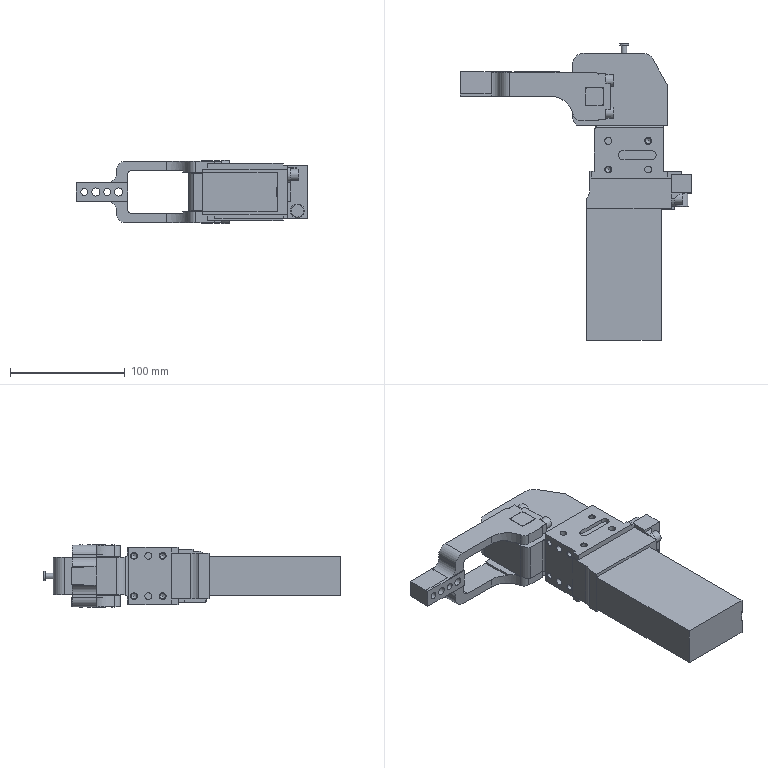Part | NX | features BREP 5 | 5 solids | 287 faces | box 202 x 258.75 x 55 mm | volume 713002 mm3 | plane 170 | cylinder 79 | cone 38 | commonest cylinder face diameters 4.917 x13 20 x12 6 x11 10 x8 8 x6 16 x4